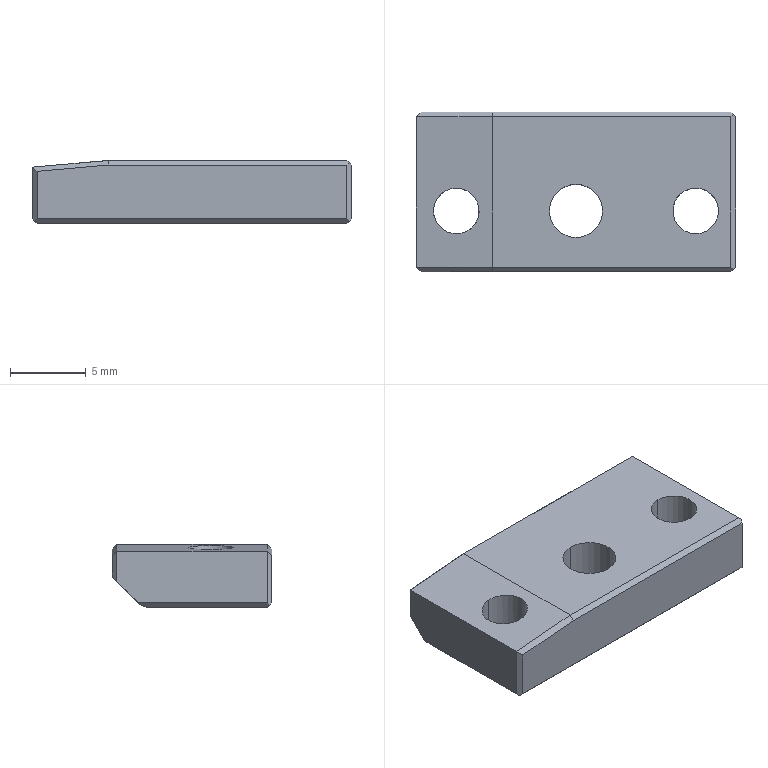Part | NX | 1 solid | 27 faces | box 21 x 10.5 x 4.15 mm | volume 759.288 mm3 | plane 21 | cylinder 6 | commonest cylinder face diameters 3 x4 3.5 x2
STEP:
#1=CARTESIAN_POINT('',(-121.3,173.5,-96.5));
#2=VERTEX_POINT('',#1);
#3=CARTESIAN_POINT('',(-137.,173.5,-96.5));
#4=VERTEX_POINT('',#3);
#5=CARTESIAN_POINT('',(-129.,173.5,-96.5));
#6=DIRECTION('',(-1.,0.,0.));
#7=VECTOR('',#6,1000.);
#8=LINE('',#5,#7);
#9=EDGE_CURVE('',#2,#4,#8,.T.);
#10=ORIENTED_EDGE('',*,*,#9,.F.);
#11=CARTESIAN_POINT('',(-121.3,183.4,-96.5));
#12=VERTEX_POINT('',#11);
#13=CARTESIAN_POINT('',(-121.3,178.45,-96.5));
#14=DIRECTION('',(0.,-1.,0.));
#15=VECTOR('',#14,1000.);
#16=LINE('',#13,#15);
#17=EDGE_CURVE('',#12,#2,#16,.T.);
#18=ORIENTED_EDGE('',*,*,#17,.F.);
#19=CARTESIAN_POINT('',(-137.,183.4,-96.5));
#20=VERTEX_POINT('',#19);
#21=CARTESIAN_POINT('',(-129.,183.4,-96.5));
#22=DIRECTION('',(-1.,0.,0.));
#23=VECTOR('',#22,1000.);
#24=LINE('',#21,#23);
#25=EDGE_CURVE('',#12,#20,#24,.T.);
#26=ORIENTED_EDGE('',*,*,#25,.T.);
#27=CARTESIAN_POINT('',(-137.,178.45,-96.5));
#28=DIRECTION('',(0.,-1.,0.));
#29=VECTOR('',#28,1000.);
#30=LINE('',#27,#29);
#31=EDGE_CURVE('',#20,#4,#30,.T.);
#32=ORIENTED_EDGE('',*,*,#31,.T.);
#33=EDGE_LOOP('',(#10,#18,#26,#32));
#34=FACE_BOUND('',#33,.T.);
#35=CARTESIAN_POINT('',(-123.625,178.7,-96.5));
#36=VERTEX_POINT('',#35);
#37=CARTESIAN_POINT('',(-123.625,175.7,-96.5));
#38=VERTEX_POINT('',#37);
#39=CARTESIAN_POINT('',(-123.625,177.2,-96.5));
#40=DIRECTION('',(0.,0.,-1.));
#41=DIRECTION('',(0.,-1.,0.));
#42=AXIS2_PLACEMENT_3D('',#39,#40,#41);
#43=CIRCLE('',#42,1.5);
#44=EDGE_CURVE('',#36,#38,#43,.T.);
#45=ORIENTED_EDGE('',*,*,#44,.T.);
#46=CARTESIAN_POINT('',(-123.625,177.2,-96.5));
#47=DIRECTION('',(0.,0.,-1.));
#48=DIRECTION('',(0.,-1.,0.));
#49=AXIS2_PLACEMENT_3D('',#46,#47,#48);
#50=CIRCLE('',#49,1.5);
#51=EDGE_CURVE('',#38,#36,#50,.T.);
#52=ORIENTED_EDGE('',*,*,#51,.T.);
#53=EDGE_LOOP('',(#45,#52));
#54=FACE_BOUND('',#53,.T.);
#55=CARTESIAN_POINT('',(-131.5,178.95,-96.5));
#56=VERTEX_POINT('',#55);
#57=CARTESIAN_POINT('',(-131.5,175.45,-96.5));
#58=VERTEX_POINT('',#57);
#59=CARTESIAN_POINT('',(-131.5,177.2,-96.5));
#60=DIRECTION('',(0.,0.,-1.));
#61=DIRECTION('',(0.,-1.,0.));
#62=AXIS2_PLACEMENT_3D('',#59,#60,#61);
#63=CIRCLE('',#62,1.75);
#64=EDGE_CURVE('',#56,#58,#63,.T.);
#65=ORIENTED_EDGE('',*,*,#64,.T.);
#66=CARTESIAN_POINT('',(-131.5,177.2,-96.5));
#67=DIRECTION('',(0.,0.,-1.));
#68=DIRECTION('',(0.,-1.,0.));
#69=AXIS2_PLACEMENT_3D('',#66,#67,#68);
#70=CIRCLE('',#69,1.75);
#71=EDGE_CURVE('',#58,#56,#70,.T.);
#72=ORIENTED_EDGE('',*,*,#71,.T.);
#73=EDGE_LOOP('',(#65,#72));
#74=FACE_BOUND('',#73,.T.);
#75=CARTESIAN_POINT('',(-121.,182.7,-96.5));
#76=DIRECTION('',(0.,0.,1.));
#77=DIRECTION('',(1.,0.,0.));
#78=AXIS2_PLACEMENT_3D('',#75,#76,#77);
#79=PLANE('',#78);
#80=ADVANCED_FACE('',(#34,#54,#74),#79,.T.);
#81=CARTESIAN_POINT('',(-141.7,183.7,-98.65));
#82=VERTEX_POINT('',#81);
#83=CARTESIAN_POINT('',(-121.3,183.7,-98.65));
#84=VERTEX_POINT('',#83);
#85=CARTESIAN_POINT('',(-131.5,183.7,-98.65));
#86=DIRECTION('',(1.,0.,0.));
#87=VECTOR('',#86,1000.);
#88=LINE('',#85,#87);
#89=EDGE_CURVE('',#82,#84,#88,.T.);
#90=ORIENTED_EDGE('',*,*,#89,.F.);
#91=CARTESIAN_POINT('',(-141.7,183.7,-97.212));
#92=VERTEX_POINT('',#91);
#93=CARTESIAN_POINT('',(-141.7,183.7,-97.944));
#94=DIRECTION('',(0.,0.,1.));
#95=VECTOR('',#94,1000.);
#96=LINE('',#93,#95);
#97=EDGE_CURVE('',#82,#92,#96,.T.);
#98=ORIENTED_EDGE('',*,*,#97,.T.);
#99=CARTESIAN_POINT('',(-136.987,183.7,-96.8));
#100=VERTEX_POINT('',#99);
#101=CARTESIAN_POINT('',(-139.474,183.7,-97.018));
#102=DIRECTION('',(0.9962,0.,0.08716));
#103=VECTOR('',#102,1000.);
#104=LINE('',#101,#103);
#105=EDGE_CURVE('',#92,#100,#104,.T.);
#106=ORIENTED_EDGE('',*,*,#105,.T.);
#107=CARTESIAN_POINT('',(-121.3,183.7,-96.8));
#108=VERTEX_POINT('',#107);
#109=CARTESIAN_POINT('',(-129.,183.7,-96.8));
#110=DIRECTION('',(-1.,0.,0.));
#111=VECTOR('',#110,1000.);
#112=LINE('',#109,#111);
#113=EDGE_CURVE('',#108,#100,#112,.T.);
#114=ORIENTED_EDGE('',*,*,#113,.F.);
#115=CARTESIAN_POINT('',(-121.3,183.7,-97.575));
#116=DIRECTION('',(0.,0.,1.));
#117=VECTOR('',#116,1000.);
#118=LINE('',#115,#117);
#119=EDGE_CURVE('',#84,#108,#118,.T.);
#120=ORIENTED_EDGE('',*,*,#119,.F.);
#121=EDGE_LOOP('',(#90,#98,#106,#114,#120));
#122=FACE_BOUND('',#121,.T.);
#123=CARTESIAN_POINT('',(-121.,183.7,-100.65));
#124=DIRECTION('',(0.,1.,0.));
#125=DIRECTION('',(1.,0.,0.));
#126=AXIS2_PLACEMENT_3D('',#123,#124,#125);
#127=PLANE('',#126);
#128=ADVANCED_FACE('',(#122),#127,.T.);
#129=CARTESIAN_POINT('',(-121.3,173.5,-100.65));
#130=VERTEX_POINT('',#129);
#131=CARTESIAN_POINT('',(-141.7,173.5,-100.65));
#132=VERTEX_POINT('',#131);
#133=CARTESIAN_POINT('',(-131.5,173.5,-100.65));
#134=DIRECTION('',(-1.,0.,0.));
#135=VECTOR('',#134,1000.);
#136=LINE('',#133,#135);
#137=EDGE_CURVE('',#130,#132,#136,.T.);
#138=ORIENTED_EDGE('',*,*,#137,.T.);
#139=CARTESIAN_POINT('',(-141.7,181.4,-100.65));
#140=VERTEX_POINT('',#139);
#141=CARTESIAN_POINT('',(-141.7,177.45,-100.65));
#142=DIRECTION('',(0.,1.,0.));
#143=VECTOR('',#142,1000.);
#144=LINE('',#141,#143);
#145=EDGE_CURVE('',#132,#140,#144,.T.);
#146=ORIENTED_EDGE('',*,*,#145,.T.);
#147=CARTESIAN_POINT('',(-121.3,181.4,-100.65));
#148=VERTEX_POINT('',#147);
#149=CARTESIAN_POINT('',(-131.5,181.4,-100.65));
#150=DIRECTION('',(1.,0.,0.));
#151=VECTOR('',#150,1000.);
#152=LINE('',#149,#151);
#153=EDGE_CURVE('',#140,#148,#152,.T.);
#154=ORIENTED_EDGE('',*,*,#153,.T.);
#155=CARTESIAN_POINT('',(-121.3,177.45,-100.65));
#156=DIRECTION('',(0.,1.,0.));
#157=VECTOR('',#156,1000.);
#158=LINE('',#155,#157);
#159=EDGE_CURVE('',#130,#148,#158,.T.);
#160=ORIENTED_EDGE('',*,*,#159,.F.);
#161=EDGE_LOOP('',(#138,#146,#154,#160));
#162=FACE_BOUND('',#161,.T.);
#163=CARTESIAN_POINT('',(-123.625,178.7,-100.65));
#164=VERTEX_POINT('',#163);
#165=CARTESIAN_POINT('',(-123.625,175.7,-100.65));
#166=VERTEX_POINT('',#165);
#167=CARTESIAN_POINT('',(-123.625,177.2,-100.65));
#168=DIRECTION('',(0.,0.,-1.));
#169=DIRECTION('',(0.,-1.,0.));
#170=AXIS2_PLACEMENT_3D('',#167,#168,#169);
#171=CIRCLE('',#170,1.5);
#172=EDGE_CURVE('',#164,#166,#171,.T.);
#173=ORIENTED_EDGE('',*,*,#172,.F.);
#174=CARTESIAN_POINT('',(-123.625,177.2,-100.65));
#175=DIRECTION('',(0.,0.,-1.));
#176=DIRECTION('',(0.,-1.,0.));
#177=AXIS2_PLACEMENT_3D('',#174,#175,#176);
#178=CIRCLE('',#177,1.5);
#179=EDGE_CURVE('',#166,#164,#178,.T.);
#180=ORIENTED_EDGE('',*,*,#179,.F.);
#181=EDGE_LOOP('',(#173,#180));
#182=FACE_BOUND('',#181,.T.);
#183=CARTESIAN_POINT('',(-139.375,178.7,-100.65));
#184=VERTEX_POINT('',#183);
#185=CARTESIAN_POINT('',(-139.375,175.7,-100.65));
#186=VERTEX_POINT('',#185);
#187=CARTESIAN_POINT('',(-139.375,177.2,-100.65));
#188=DIRECTION('',(0.,0.,-1.));
#189=DIRECTION('',(0.,-1.,0.));
#190=AXIS2_PLACEMENT_3D('',#187,#188,#189);
#191=CIRCLE('',#190,1.5);
#192=EDGE_CURVE('',#184,#186,#191,.T.);
#193=ORIENTED_EDGE('',*,*,#192,.F.);
#194=CARTESIAN_POINT('',(-139.375,177.2,-100.65));
#195=DIRECTION('',(0.,0.,-1.));
#196=DIRECTION('',(0.,-1.,0.));
#197=AXIS2_PLACEMENT_3D('',#194,#195,#196);
#198=CIRCLE('',#197,1.5);
#199=EDGE_CURVE('',#186,#184,#198,.T.);
#200=ORIENTED_EDGE('',*,*,#199,.F.);
#201=EDGE_LOOP('',(#193,#200));
#202=FACE_BOUND('',#201,.T.);
#203=CARTESIAN_POINT('',(-131.5,178.95,-100.65));
#204=VERTEX_POINT('',#203);
#205=CARTESIAN_POINT('',(-131.5,175.45,-100.65));
#206=VERTEX_POINT('',#205);
#207=CARTESIAN_POINT('',(-131.5,177.2,-100.65));
#208=DIRECTION('',(0.,0.,-1.));
#209=DIRECTION('',(0.,-1.,0.));
#210=AXIS2_PLACEMENT_3D('',#207,#208,#209);
#211=CIRCLE('',#210,1.75);
#212=EDGE_CURVE('',#204,#206,#211,.T.);
#213=ORIENTED_EDGE('',*,*,#212,.F.);
#214=CARTESIAN_POINT('',(-131.5,177.2,-100.65));
#215=DIRECTION('',(0.,0.,-1.));
#216=DIRECTION('',(0.,-1.,0.));
#217=AXIS2_PLACEMENT_3D('',#214,#215,#216);
#218=CIRCLE('',#217,1.75);
#219=EDGE_CURVE('',#206,#204,#218,.T.);
#220=ORIENTED_EDGE('',*,*,#219,.F.);
#221=EDGE_LOOP('',(#213,#220));
#222=FACE_BOUND('',#221,.T.);
#223=CARTESIAN_POINT('',(-121.,173.2,-100.65));
#224=DIRECTION('',(0.,0.,-1.));
#225=DIRECTION('',(0.,-1.,0.));
#226=AXIS2_PLACEMENT_3D('',#223,#224,#225);
#227=PLANE('',#226);
#228=ADVANCED_FACE('',(#162,#182,#202,#222),#227,.T.);
#229=CARTESIAN_POINT('',(-121.3,173.2,-96.8));
#230=VERTEX_POINT('',#229);
#231=CARTESIAN_POINT('',(-121.3,173.2,-100.35));
#232=VERTEX_POINT('',#231);
#233=CARTESIAN_POINT('',(-121.3,173.2,-98.575));
#234=DIRECTION('',(0.,0.,-1.));
#235=VECTOR('',#234,1000.);
#236=LINE('',#233,#235);
#237=EDGE_CURVE('',#230,#232,#236,.T.);
#238=ORIENTED_EDGE('',*,*,#237,.F.);
#239=CARTESIAN_POINT('',(-136.987,173.2,-96.8));
#240=VERTEX_POINT('',#239);
#241=CARTESIAN_POINT('',(-129.,173.2,-96.8));
#242=DIRECTION('',(-1.,0.,0.));
#243=VECTOR('',#242,1000.);
#244=LINE('',#241,#243);
#245=EDGE_CURVE('',#230,#240,#244,.T.);
#246=ORIENTED_EDGE('',*,*,#245,.T.);
#247=CARTESIAN_POINT('',(-141.7,173.2,-97.212));
#248=VERTEX_POINT('',#247);
#249=CARTESIAN_POINT('',(-139.474,173.2,-97.018));
#250=DIRECTION('',(-0.9962,0.,-0.08716));
#251=VECTOR('',#250,1000.);
#252=LINE('',#249,#251);
#253=EDGE_CURVE('',#240,#248,#252,.T.);
#254=ORIENTED_EDGE('',*,*,#253,.T.);
#255=CARTESIAN_POINT('',(-141.7,173.2,-100.35));
#256=VERTEX_POINT('',#255);
#257=CARTESIAN_POINT('',(-141.7,173.2,-98.794));
#258=DIRECTION('',(0.,0.,-1.));
#259=VECTOR('',#258,1000.);
#260=LINE('',#257,#259);
#261=EDGE_CURVE('',#248,#256,#260,.T.);
#262=ORIENTED_EDGE('',*,*,#261,.T.);
#263=CARTESIAN_POINT('',(-131.5,173.2,-100.35));
#264=DIRECTION('',(-1.,0.,0.));
#265=VECTOR('',#264,1000.);
#266=LINE('',#263,#265);
#267=EDGE_CURVE('',#232,#256,#266,.T.);
#268=ORIENTED_EDGE('',*,*,#267,.F.);
#269=EDGE_LOOP('',(#238,#246,#254,#262,#268));
#270=FACE_BOUND('',#269,.T.);
#271=CARTESIAN_POINT('',(-121.,173.2,-96.5));
#272=DIRECTION('',(0.,-1.,0.));
#273=DIRECTION('',(0.,0.,-1.));
#274=AXIS2_PLACEMENT_3D('',#271,#272,#273);
#275=PLANE('',#274);
#276=ADVANCED_FACE('',(#270),#275,.T.);
#277=CARTESIAN_POINT('',(-141.912,181.912,-100.438));
#278=VERTEX_POINT('',#277);
#279=CARTESIAN_POINT('',(-121.088,181.912,-100.438));
#280=VERTEX_POINT('',#279);
#281=CARTESIAN_POINT('',(-131.5,181.912,-100.438));
#282=DIRECTION('',(1.,0.,0.));
#283=VECTOR('',#282,1000.);
#284=LINE('',#281,#283);
#285=EDGE_CURVE('',#278,#280,#284,.T.);
#286=ORIENTED_EDGE('',*,*,#285,.F.);
#287=CARTESIAN_POINT('',(-142.,182.,-100.35));
#288=VERTEX_POINT('',#287);
#289=CARTESIAN_POINT('',(-121.,161.,-121.35));
#290=DIRECTION('',(0.5774,-0.5774,-0.5774));
#291=VECTOR('',#290,1000.);
#292=LINE('',#289,#291);
#293=EDGE_CURVE('',#288,#278,#292,.T.);
#294=ORIENTED_EDGE('',*,*,#293,.F.);
#295=CARTESIAN_POINT('',(-142.,183.4,-98.95));
#296=VERTEX_POINT('',#295);
#297=CARTESIAN_POINT('',(-142.,196.267,-86.083));
#298=DIRECTION('',(0.,0.7071,0.7071));
#299=VECTOR('',#298,1000.);
#300=LINE('',#297,#299);
#301=EDGE_CURVE('',#288,#296,#300,.T.);
#302=ORIENTED_EDGE('',*,*,#301,.T.);
#303=CARTESIAN_POINT('',(-121.,204.4,-77.95));
#304=DIRECTION('',(-0.5774,-0.5774,-0.5774));
#305=VECTOR('',#304,1000.);
#306=LINE('',#303,#305);
#307=EDGE_CURVE('',#82,#296,#306,.T.);
#308=ORIENTED_EDGE('',*,*,#307,.F.);
#309=ORIENTED_EDGE('',*,*,#89,.T.);
#310=CARTESIAN_POINT('',(-121.,183.4,-98.95));
#311=VERTEX_POINT('',#310);
#312=CARTESIAN_POINT('',(-121.,183.4,-98.95));
#313=DIRECTION('',(0.5774,-0.5774,-0.5774));
#314=VECTOR('',#313,1000.);
#315=LINE('',#312,#314);
#316=EDGE_CURVE('',#84,#311,#315,.T.);
#317=ORIENTED_EDGE('',*,*,#316,.T.);
#318=CARTESIAN_POINT('',(-121.,182.,-100.35));
#319=VERTEX_POINT('',#318);
#320=CARTESIAN_POINT('',(-121.,196.267,-86.083));
#321=DIRECTION('',(0.,0.7071,0.7071));
#322=VECTOR('',#321,1000.);
#323=LINE('',#320,#322);
#324=EDGE_CURVE('',#319,#311,#323,.T.);
#325=ORIENTED_EDGE('',*,*,#324,.F.);
#326=CARTESIAN_POINT('',(-106.733,196.267,-86.083));
#327=DIRECTION('',(-0.5774,-0.5774,-0.5774));
#328=VECTOR('',#327,1000.);
#329=LINE('',#326,#328);
#330=EDGE_CURVE('',#319,#280,#329,.T.);
#331=ORIENTED_EDGE('',*,*,#330,.T.);
#332=EDGE_LOOP('',(#286,#294,#302,#308,#309,#317,#325,#331));
#333=FACE_BOUND('',#332,.T.);
#334=CARTESIAN_POINT('',(-131.5,182.7,-99.65));
#335=DIRECTION('',(0.,-0.7071,0.7071));
#336=DIRECTION('',(-1.,0.,0.));
#337=AXIS2_PLACEMENT_3D('',#334,#335,#336);
#338=PLANE('',#337);
#339=ADVANCED_FACE('',(#333),#338,.F.);
#340=ORIENTED_EDGE('',*,*,#64,.F.);
#341=CARTESIAN_POINT('',(-131.5,178.95,-96.085));
#342=DIRECTION('',(0.,0.,-1.));
#343=VECTOR('',#342,1000.);
#344=LINE('',#341,#343);
#345=EDGE_CURVE('',#204,#56,#344,.F.);
#346=ORIENTED_EDGE('',*,*,#345,.F.);
#347=ORIENTED_EDGE('',*,*,#212,.T.);
#348=CARTESIAN_POINT('',(-131.5,175.45,-96.085));
#349=DIRECTION('',(0.,0.,-1.));
#350=VECTOR('',#349,1000.);
#351=LINE('',#348,#350);
#352=EDGE_CURVE('',#206,#58,#351,.F.);
#353=ORIENTED_EDGE('',*,*,#352,.T.);
#354=EDGE_LOOP('',(#340,#346,#347,#353));
#355=FACE_BOUND('',#354,.T.);
#356=CARTESIAN_POINT('',(-131.5,177.2,-96.085));
#357=DIRECTION('',(0.,0.,-1.));
#358=DIRECTION('',(0.,-1.,0.));
#359=AXIS2_PLACEMENT_3D('',#356,#357,#358);
#360=CYLINDRICAL_SURFACE('',#359,1.75);
#361=ADVANCED_FACE('',(#355),#360,.F.);
#362=ORIENTED_EDGE('',*,*,#44,.F.);
#363=CARTESIAN_POINT('',(-123.625,178.7,-96.085));
#364=DIRECTION('',(0.,0.,-1.));
#365=VECTOR('',#364,1000.);
#366=LINE('',#363,#365);
#367=EDGE_CURVE('',#164,#36,#366,.F.);
#368=ORIENTED_EDGE('',*,*,#367,.F.);
#369=ORIENTED_EDGE('',*,*,#172,.T.);
#370=CARTESIAN_POINT('',(-123.625,175.7,-96.085));
#371=DIRECTION('',(0.,0.,-1.));
#372=VECTOR('',#371,1000.);
#373=LINE('',#370,#372);
#374=EDGE_CURVE('',#166,#38,#373,.F.);
#375=ORIENTED_EDGE('',*,*,#374,.T.);
#376=EDGE_LOOP('',(#362,#368,#369,#375));
#377=FACE_BOUND('',#376,.T.);
#378=CARTESIAN_POINT('',(-123.625,177.2,-96.085));
#379=DIRECTION('',(0.,0.,-1.));
#380=DIRECTION('',(0.,-1.,0.));
#381=AXIS2_PLACEMENT_3D('',#378,#379,#380);
#382=CYLINDRICAL_SURFACE('',#381,1.5);
#383=ADVANCED_FACE('',(#377),#382,.F.);
#384=CARTESIAN_POINT('',(-139.375,178.7,-96.708));
#385=VERTEX_POINT('',#384);
#386=CARTESIAN_POINT('',(-139.375,175.7,-96.708));
#387=VERTEX_POINT('',#386);
#388=CARTESIAN_POINT('',(-139.375,178.7,-96.708));
#389=CARTESIAN_POINT('',(-136.375,178.7,-96.445));
#390=CARTESIAN_POINT('',(-136.375,175.7,-96.445));
#391=CARTESIAN_POINT('',(-139.375,175.7,-96.708));
#392=(BOUNDED_CURVE()B_SPLINE_CURVE(3,(#388,#389,#390,#391),.UNSPECIFIED.,.F.,.F.)B_SPLINE_CURVE_WITH_KNOTS((4,4),(4.712,7.854),.UNSPECIFIED.)CURVE()GEOMETRIC_REPRESENTATION_ITEM()RATIONAL_B_SPLINE_CURVE((1.,0.3333,0.3333,1.))REPRESENTATION_ITEM(''));
#393=EDGE_CURVE('',#385,#387,#392,.T.);
#394=ORIENTED_EDGE('',*,*,#393,.F.);
#395=CARTESIAN_POINT('',(-139.375,178.7,-96.085));
#396=DIRECTION('',(0.,0.,-1.));
#397=VECTOR('',#396,1000.);
#398=LINE('',#395,#397);
#399=EDGE_CURVE('',#184,#385,#398,.F.);
#400=ORIENTED_EDGE('',*,*,#399,.F.);
#401=ORIENTED_EDGE('',*,*,#192,.T.);
#402=CARTESIAN_POINT('',(-139.375,175.7,-96.085));
#403=DIRECTION('',(0.,0.,-1.));
#404=VECTOR('',#403,1000.);
#405=LINE('',#402,#404);
#406=EDGE_CURVE('',#186,#387,#405,.F.);
#407=ORIENTED_EDGE('',*,*,#406,.T.);
#408=EDGE_LOOP('',(#394,#400,#401,#407));
#409=FACE_BOUND('',#408,.T.);
#410=CARTESIAN_POINT('',(-139.375,177.2,-96.085));
#411=DIRECTION('',(0.,0.,-1.));
#412=DIRECTION('',(0.,-1.,0.));
#413=AXIS2_PLACEMENT_3D('',#410,#411,#412);
#414=CYLINDRICAL_SURFACE('',#413,1.5);
#415=ADVANCED_FACE('',(#409),#414,.F.);
#416=ORIENTED_EDGE('',*,*,#25,.F.);
#417=CARTESIAN_POINT('',(-121.15,183.55,-96.65));
#418=VERTEX_POINT('',#417);
#419=CARTESIAN_POINT('',(-131.717,172.983,-86.083));
#420=DIRECTION('',(0.5774,0.5774,-0.5774));
#421=VECTOR('',#420,1000.);
#422=LINE('',#419,#421);
#423=EDGE_CURVE('',#12,#418,#422,.T.);
#424=ORIENTED_EDGE('',*,*,#423,.T.);
#425=CARTESIAN_POINT('',(-110.583,172.983,-86.083));
#426=DIRECTION('',(-0.5774,0.5774,-0.5774));
#427=VECTOR('',#426,1000.);
#428=LINE('',#425,#427);
#429=EDGE_CURVE('',#418,#108,#428,.T.);
#430=ORIENTED_EDGE('',*,*,#429,.T.);
#431=ORIENTED_EDGE('',*,*,#113,.T.);
#432=CARTESIAN_POINT('',(-137.455,172.983,-86.083));
#433=DIRECTION('',(0.03086,0.7068,-0.7068));
#434=VECTOR('',#433,1000.);
#435=LINE('',#432,#434);
#436=EDGE_CURVE('',#20,#100,#435,.T.);
#437=ORIENTED_EDGE('',*,*,#436,.F.);
#438=EDGE_LOOP('',(#416,#424,#430,#431,#437));
#439=FACE_BOUND('',#438,.T.);
#440=CARTESIAN_POINT('',(-129.,183.55,-96.65));
#441=DIRECTION('',(0.,0.7071,0.7071));
#442=DIRECTION('',(1.,0.,0.));
#443=AXIS2_PLACEMENT_3D('',#440,#441,#442);
#444=PLANE('',#443);
#445=ADVANCED_FACE('',(#439),#444,.T.);
#446=ORIENTED_EDGE('',*,*,#285,.T.);
#447=CARTESIAN_POINT('',(-122.939,177.442,-102.289));
#448=DIRECTION('',(0.3574,0.8629,0.3574));
#449=VECTOR('',#448,1000.);
#450=LINE('',#447,#449);
#451=EDGE_CURVE('',#148,#280,#450,.T.);
#452=ORIENTED_EDGE('',*,*,#451,.F.);
#453=ORIENTED_EDGE('',*,*,#153,.F.);
#454=CARTESIAN_POINT('',(-140.061,177.442,-102.289));
#455=DIRECTION('',(-0.3574,0.8629,0.3574));
#456=VECTOR('',#455,1000.);
#457=LINE('',#454,#456);
#458=EDGE_CURVE('',#140,#278,#457,.T.);
#459=ORIENTED_EDGE('',*,*,#458,.T.);
#460=EDGE_LOOP('',(#446,#452,#453,#459));
#461=FACE_BOUND('',#460,.T.);
#462=CARTESIAN_POINT('',(-131.5,181.656,-100.544));
#463=DIRECTION('',(0.,-0.3827,0.9239));
#464=DIRECTION('',(-1.,0.,0.));
#465=AXIS2_PLACEMENT_3D('',#462,#463,#464);
#466=PLANE('',#465);
#467=ADVANCED_FACE('',(#461),#466,.F.);
#468=ORIENTED_EDGE('',*,*,#137,.F.);
#469=CARTESIAN_POINT('',(-121.15,173.35,-100.5));
#470=VERTEX_POINT('',#469);
#471=CARTESIAN_POINT('',(-106.733,158.933,-86.083));
#472=DIRECTION('',(0.5774,-0.5774,0.5774));
#473=VECTOR('',#472,1000.);
#474=LINE('',#471,#473);
#475=EDGE_CURVE('',#130,#470,#474,.T.);
#476=ORIENTED_EDGE('',*,*,#475,.T.);
#477=CARTESIAN_POINT('',(-135.567,158.933,-86.083));
#478=DIRECTION('',(-0.5774,-0.5774,0.5774));
#479=VECTOR('',#478,1000.);
#480=LINE('',#477,#479);
#481=EDGE_CURVE('',#470,#232,#480,.T.);
#482=ORIENTED_EDGE('',*,*,#481,.T.);
#483=ORIENTED_EDGE('',*,*,#267,.T.);
#484=CARTESIAN_POINT('',(-141.85,173.35,-100.5));
#485=VERTEX_POINT('',#484);
#486=CARTESIAN_POINT('',(-121.,152.5,-79.65));
#487=DIRECTION('',(-0.5774,0.5774,-0.5774));
#488=VECTOR('',#487,1000.);
#489=LINE('',#486,#488);
#490=EDGE_CURVE('',#256,#485,#489,.T.);
#491=ORIENTED_EDGE('',*,*,#490,.T.);
#492=CARTESIAN_POINT('',(-121.,194.2,-121.35));
#493=DIRECTION('',(0.5774,0.5774,-0.5774));
#494=VECTOR('',#493,1000.);
#495=LINE('',#492,#494);
#496=EDGE_CURVE('',#485,#132,#495,.T.);
#497=ORIENTED_EDGE('',*,*,#496,.T.);
#498=EDGE_LOOP('',(#468,#476,#482,#483,#491,#497));
#499=FACE_BOUND('',#498,.T.);
#500=CARTESIAN_POINT('',(-131.5,173.35,-100.5));
#501=DIRECTION('',(0.,-0.7071,-0.7071));
#502=DIRECTION('',(0.,0.7071,-0.7071));
#503=AXIS2_PLACEMENT_3D('',#500,#501,#502);
#504=PLANE('',#503);
#505=ADVANCED_FACE('',(#499),#504,.T.);
#506=ORIENTED_EDGE('',*,*,#9,.T.);
#507=CARTESIAN_POINT('',(-137.455,183.917,-86.083));
#508=DIRECTION('',(0.03086,-0.7068,-0.7068));
#509=VECTOR('',#508,1000.);
#510=LINE('',#507,#509);
#511=EDGE_CURVE('',#4,#240,#510,.T.);
#512=ORIENTED_EDGE('',*,*,#511,.T.);
#513=ORIENTED_EDGE('',*,*,#245,.F.);
#514=CARTESIAN_POINT('',(-121.15,173.35,-96.65));
#515=VERTEX_POINT('',#514);
#516=CARTESIAN_POINT('',(-121.,173.5,-96.5));
#517=DIRECTION('',(-0.5774,-0.5774,-0.5774));
#518=VECTOR('',#517,1000.);
#519=LINE('',#516,#518);
#520=EDGE_CURVE('',#515,#230,#519,.T.);
#521=ORIENTED_EDGE('',*,*,#520,.F.);
#522=CARTESIAN_POINT('',(-131.717,183.917,-86.083));
#523=DIRECTION('',(0.5774,-0.5774,-0.5774));
#524=VECTOR('',#523,1000.);
#525=LINE('',#522,#524);
#526=EDGE_CURVE('',#2,#515,#525,.T.);
#527=ORIENTED_EDGE('',*,*,#526,.F.);
#528=EDGE_LOOP('',(#506,#512,#513,#521,#527));
#529=FACE_BOUND('',#528,.T.);
#530=CARTESIAN_POINT('',(-129.,173.35,-96.65));
#531=DIRECTION('',(0.,0.7071,-0.7071));
#532=DIRECTION('',(-1.,0.,0.));
#533=AXIS2_PLACEMENT_3D('',#530,#531,#532);
#534=PLANE('',#533);
#535=ADVANCED_FACE('',(#529),#534,.F.);
#536=ORIENTED_EDGE('',*,*,#406,.F.);
#537=ORIENTED_EDGE('',*,*,#199,.T.);
#538=ORIENTED_EDGE('',*,*,#399,.T.);
#539=CARTESIAN_POINT('',(-139.375,175.7,-96.708));
#540=CARTESIAN_POINT('',(-142.375,175.7,-96.97));
#541=CARTESIAN_POINT('',(-142.375,178.7,-96.97));
#542=CARTESIAN_POINT('',(-139.375,178.7,-96.708));
#543=(BOUNDED_CURVE()B_SPLINE_CURVE(3,(#539,#540,#541,#542),.UNSPECIFIED.,.F.,.F.)B_SPLINE_CURVE_WITH_KNOTS((4,4),(1.571,4.712),.UNSPECIFIED.)CURVE()GEOMETRIC_REPRESENTATION_ITEM()RATIONAL_B_SPLINE_CURVE((1.,0.3333,0.3333,1.))REPRESENTATION_ITEM(''));
#544=EDGE_CURVE('',#387,#385,#543,.T.);
#545=ORIENTED_EDGE('',*,*,#544,.F.);
#546=EDGE_LOOP('',(#536,#537,#538,#545));
#547=FACE_BOUND('',#546,.T.);
#548=CARTESIAN_POINT('',(-139.375,177.2,-96.085));
#549=DIRECTION('',(0.,0.,-1.));
#550=DIRECTION('',(0.,-1.,0.));
#551=AXIS2_PLACEMENT_3D('',#548,#549,#550);
#552=CYLINDRICAL_SURFACE('',#551,1.5);
#553=ADVANCED_FACE('',(#547),#552,.F.);
#554=ORIENTED_EDGE('',*,*,#374,.F.);
#555=ORIENTED_EDGE('',*,*,#179,.T.);
#556=ORIENTED_EDGE('',*,*,#367,.T.);
#557=ORIENTED_EDGE('',*,*,#51,.F.);
#558=EDGE_LOOP('',(#554,#555,#556,#557));
#559=FACE_BOUND('',#558,.T.);
#560=CARTESIAN_POINT('',(-123.625,177.2,-96.085));
#561=DIRECTION('',(0.,0.,-1.));
#562=DIRECTION('',(0.,-1.,0.));
#563=AXIS2_PLACEMENT_3D('',#560,#561,#562);
#564=CYLINDRICAL_SURFACE('',#563,1.5);
#565=ADVANCED_FACE('',(#559),#564,.F.);
#566=ORIENTED_EDGE('',*,*,#352,.F.);
#567=ORIENTED_EDGE('',*,*,#219,.T.);
#568=ORIENTED_EDGE('',*,*,#345,.T.);
#569=ORIENTED_EDGE('',*,*,#71,.F.);
#570=EDGE_LOOP('',(#566,#567,#568,#569));
#571=FACE_BOUND('',#570,.T.);
#572=CARTESIAN_POINT('',(-131.5,177.2,-96.085));
#573=DIRECTION('',(0.,0.,-1.));
#574=DIRECTION('',(0.,-1.,0.));
#575=AXIS2_PLACEMENT_3D('',#572,#573,#574);
#576=CYLINDRICAL_SURFACE('',#575,1.75);
#577=ADVANCED_FACE('',(#571),#576,.F.);
#578=CARTESIAN_POINT('',(-142.,183.4,-96.937));
#579=VERTEX_POINT('',#578);
#580=CARTESIAN_POINT('',(-142.,183.4,-97.944));
#581=DIRECTION('',(0.,0.,1.));
#582=VECTOR('',#581,1000.);
#583=LINE('',#580,#582);
#584=EDGE_CURVE('',#296,#579,#583,.T.);
#585=ORIENTED_EDGE('',*,*,#584,.F.);
#586=ORIENTED_EDGE('',*,*,#301,.F.);
#587=CARTESIAN_POINT('',(-142.,173.5,-100.35));
#588=VERTEX_POINT('',#587);
#589=CARTESIAN_POINT('',(-142.,177.45,-100.35));
#590=DIRECTION('',(0.,1.,0.));
#591=VECTOR('',#590,1000.);
#592=LINE('',#589,#591);
#593=EDGE_CURVE('',#588,#288,#592,.T.);
#594=ORIENTED_EDGE('',*,*,#593,.F.);
#595=CARTESIAN_POINT('',(-142.,173.5,-96.937));
#596=VERTEX_POINT('',#595);
#597=CARTESIAN_POINT('',(-142.,173.5,-98.794));
#598=DIRECTION('',(0.,0.,-1.));
#599=VECTOR('',#598,1000.);
#600=LINE('',#597,#599);
#601=EDGE_CURVE('',#596,#588,#600,.T.);
#602=ORIENTED_EDGE('',*,*,#601,.F.);
#603=CARTESIAN_POINT('',(-142.,178.45,-96.937));
#604=DIRECTION('',(0.,-1.,0.));
#605=VECTOR('',#604,1000.);
#606=LINE('',#603,#605);
#607=EDGE_CURVE('',#579,#596,#606,.T.);
#608=ORIENTED_EDGE('',*,*,#607,.F.);
#609=EDGE_LOOP('',(#585,#586,#594,#602,#608));
#610=FACE_BOUND('',#609,.T.);
#611=CARTESIAN_POINT('',(-142.,177.442,-86.083));
#612=DIRECTION('',(1.,0.,0.));
#613=DIRECTION('',(0.,1.,0.));
#614=AXIS2_PLACEMENT_3D('',#611,#612,#613);
#615=PLANE('',#614);
#616=ADVANCED_FACE('',(#610),#615,.F.);
#617=CARTESIAN_POINT('',(-139.5,173.5,-96.719));
#618=DIRECTION('',(-0.9962,0.,-0.08716));
#619=VECTOR('',#618,1000.);
#620=LINE('',#617,#619);
#621=EDGE_CURVE('',#4,#596,#620,.T.);
#622=ORIENTED_EDGE('',*,*,#621,.F.);
#623=ORIENTED_EDGE('',*,*,#31,.F.);
#624=CARTESIAN_POINT('',(-139.5,183.4,-96.719));
#625=DIRECTION('',(0.9962,0.,0.08716));
#626=VECTOR('',#625,1000.);
#627=LINE('',#624,#626);
#628=EDGE_CURVE('',#579,#20,#627,.T.);
#629=ORIENTED_EDGE('',*,*,#628,.F.);
#630=ORIENTED_EDGE('',*,*,#607,.T.);
#631=EDGE_LOOP('',(#622,#623,#629,#630));
#632=FACE_BOUND('',#631,.T.);
#633=ORIENTED_EDGE('',*,*,#393,.T.);
#634=ORIENTED_EDGE('',*,*,#544,.T.);
#635=EDGE_LOOP('',(#633,#634));
#636=FACE_BOUND('',#635,.T.);
#637=CARTESIAN_POINT('',(-139.5,178.45,-96.719));
#638=DIRECTION('',(0.08716,0.,-0.9962));
#639=DIRECTION('',(0.,-1.,0.));
#640=AXIS2_PLACEMENT_3D('',#637,#638,#639);
#641=PLANE('',#640);
#642=ADVANCED_FACE('',(#632,#636),#641,.F.);
#643=ORIENTED_EDGE('',*,*,#628,.T.);
#644=ORIENTED_EDGE('',*,*,#436,.T.);
#645=ORIENTED_EDGE('',*,*,#105,.F.);
#646=CARTESIAN_POINT('',(-121.,204.4,-116.18));
#647=DIRECTION('',(0.5934,0.5934,-0.5438));
#648=VECTOR('',#647,1000.);
#649=LINE('',#646,#648);
#650=EDGE_CURVE('',#579,#92,#649,.T.);
#651=ORIENTED_EDGE('',*,*,#650,.F.);
#652=EDGE_LOOP('',(#643,#644,#645,#651));
#653=FACE_BOUND('',#652,.T.);
#654=CARTESIAN_POINT('',(-139.487,183.55,-96.868));
#655=DIRECTION('',(0.06163,-0.7071,-0.7044));
#656=DIRECTION('',(0.,0.7058,-0.7085));
#657=AXIS2_PLACEMENT_3D('',#654,#655,#656);
#658=PLANE('',#657);
#659=ADVANCED_FACE('',(#653),#658,.F.);
#660=ORIENTED_EDGE('',*,*,#593,.T.);
#661=ORIENTED_EDGE('',*,*,#293,.T.);
#662=ORIENTED_EDGE('',*,*,#458,.F.);
#663=ORIENTED_EDGE('',*,*,#145,.F.);
#664=ORIENTED_EDGE('',*,*,#496,.F.);
#665=CARTESIAN_POINT('',(-156.267,187.767,-86.083));
#666=DIRECTION('',(-0.5774,0.5774,0.5774));
#667=VECTOR('',#666,1000.);
#668=LINE('',#665,#667);
#669=EDGE_CURVE('',#485,#588,#668,.T.);
#670=ORIENTED_EDGE('',*,*,#669,.T.);
#671=EDGE_LOOP('',(#660,#661,#662,#663,#664,#670));
#672=FACE_BOUND('',#671,.T.);
#673=CARTESIAN_POINT('',(-141.85,177.45,-100.5));
#674=DIRECTION('',(0.7071,0.,0.7071));
#675=DIRECTION('',(0.,-1.,0.));
#676=AXIS2_PLACEMENT_3D('',#673,#674,#675);
#677=PLANE('',#676);
#678=ADVANCED_FACE('',(#672),#677,.F.);
#679=ORIENTED_EDGE('',*,*,#601,.T.);
#680=ORIENTED_EDGE('',*,*,#669,.F.);
#681=ORIENTED_EDGE('',*,*,#490,.F.);
#682=ORIENTED_EDGE('',*,*,#261,.F.);
#683=CARTESIAN_POINT('',(-121.,152.5,-116.18));
#684=DIRECTION('',(-0.5934,0.5934,0.5438));
#685=VECTOR('',#684,1000.);
#686=LINE('',#683,#685);
#687=EDGE_CURVE('',#248,#596,#686,.T.);
#688=ORIENTED_EDGE('',*,*,#687,.T.);
#689=EDGE_LOOP('',(#679,#680,#681,#682,#688));
#690=FACE_BOUND('',#689,.T.);
#691=CARTESIAN_POINT('',(-141.85,173.35,-98.794));
#692=DIRECTION('',(0.7071,0.7071,0.));
#693=DIRECTION('',(0.,0.,-1.));
#694=AXIS2_PLACEMENT_3D('',#691,#692,#693);
#695=PLANE('',#694);
#696=ADVANCED_FACE('',(#690),#695,.F.);
#697=ORIENTED_EDGE('',*,*,#621,.T.);
#698=ORIENTED_EDGE('',*,*,#687,.F.);
#699=ORIENTED_EDGE('',*,*,#253,.F.);
#700=ORIENTED_EDGE('',*,*,#511,.F.);
#701=EDGE_LOOP('',(#697,#698,#699,#700));
#702=FACE_BOUND('',#701,.T.);
#703=CARTESIAN_POINT('',(-139.487,173.35,-96.868));
#704=DIRECTION('',(0.06163,0.7071,-0.7044));
#705=DIRECTION('',(-0.9962,0.,-0.08716));
#706=AXIS2_PLACEMENT_3D('',#703,#704,#705);
#707=PLANE('',#706);
#708=ADVANCED_FACE('',(#702),#707,.F.);
#709=ORIENTED_EDGE('',*,*,#584,.T.);
#710=ORIENTED_EDGE('',*,*,#650,.T.);
#711=ORIENTED_EDGE('',*,*,#97,.F.);
#712=ORIENTED_EDGE('',*,*,#307,.T.);
#713=EDGE_LOOP('',(#709,#710,#711,#712));
#714=FACE_BOUND('',#713,.T.);
#715=CARTESIAN_POINT('',(-141.85,183.55,-97.944));
#716=DIRECTION('',(0.7071,-0.7071,0.));
#717=DIRECTION('',(0.,0.,-1.));
#718=AXIS2_PLACEMENT_3D('',#715,#716,#717);
#719=PLANE('',#718);
#720=ADVANCED_FACE('',(#714),#719,.F.);
#721=CARTESIAN_POINT('',(-121.,183.4,-96.8));
#722=VERTEX_POINT('',#721);
#723=CARTESIAN_POINT('',(-121.,183.4,-97.575));
#724=DIRECTION('',(0.,0.,1.));
#725=VECTOR('',#724,1000.);
#726=LINE('',#723,#725);
#727=EDGE_CURVE('',#311,#722,#726,.T.);
#728=ORIENTED_EDGE('',*,*,#727,.T.);
#729=CARTESIAN_POINT('',(-121.,173.5,-96.8));
#730=VERTEX_POINT('',#729);
#731=CARTESIAN_POINT('',(-121.,178.45,-96.8));
#732=DIRECTION('',(0.,-1.,0.));
#733=VECTOR('',#732,1000.);
#734=LINE('',#731,#733);
#735=EDGE_CURVE('',#722,#730,#734,.T.);
#736=ORIENTED_EDGE('',*,*,#735,.T.);
#737=CARTESIAN_POINT('',(-121.,173.5,-100.35));
#738=VERTEX_POINT('',#737);
#739=CARTESIAN_POINT('',(-121.,173.5,-98.575));
#740=DIRECTION('',(0.,0.,-1.));
#741=VECTOR('',#740,1000.);
#742=LINE('',#739,#741);
#743=EDGE_CURVE('',#730,#738,#742,.T.);
#744=ORIENTED_EDGE('',*,*,#743,.T.);
#745=CARTESIAN_POINT('',(-121.,177.45,-100.35));
#746=DIRECTION('',(0.,1.,0.));
#747=VECTOR('',#746,1000.);
#748=LINE('',#745,#747);
#749=EDGE_CURVE('',#738,#319,#748,.T.);
#750=ORIENTED_EDGE('',*,*,#749,.T.);
#751=ORIENTED_EDGE('',*,*,#324,.T.);
#752=EDGE_LOOP('',(#728,#736,#744,#750,#751));
#753=FACE_BOUND('',#752,.T.);
#754=CARTESIAN_POINT('',(-121.,177.442,-86.083));
#755=DIRECTION('',(1.,0.,0.));
#756=DIRECTION('',(0.,1.,0.));
#757=AXIS2_PLACEMENT_3D('',#754,#755,#756);
#758=PLANE('',#757);
#759=ADVANCED_FACE('',(#753),#758,.T.);
#760=ORIENTED_EDGE('',*,*,#743,.F.);
#761=CARTESIAN_POINT('',(-131.717,162.783,-86.083));
#762=DIRECTION('',(-0.5774,-0.5774,0.5774));
#763=VECTOR('',#762,1000.);
#764=LINE('',#761,#763);
#765=EDGE_CURVE('',#730,#515,#764,.T.);
#766=ORIENTED_EDGE('',*,*,#765,.T.);
#767=ORIENTED_EDGE('',*,*,#520,.T.);
#768=ORIENTED_EDGE('',*,*,#237,.T.);
#769=ORIENTED_EDGE('',*,*,#481,.F.);
#770=CARTESIAN_POINT('',(-106.733,187.767,-86.083));
#771=DIRECTION('',(0.5774,0.5774,0.5774));
#772=VECTOR('',#771,1000.);
#773=LINE('',#770,#772);
#774=EDGE_CURVE('',#470,#738,#773,.T.);
#775=ORIENTED_EDGE('',*,*,#774,.T.);
#776=EDGE_LOOP('',(#760,#766,#767,#768,#769,#775));
#777=FACE_BOUND('',#776,.T.);
#778=CARTESIAN_POINT('',(-121.15,173.35,-98.575));
#779=DIRECTION('',(0.7071,-0.7071,0.));
#780=DIRECTION('',(0.,0.,-1.));
#781=AXIS2_PLACEMENT_3D('',#778,#779,#780);
#782=PLANE('',#781);
#783=ADVANCED_FACE('',(#777),#782,.T.);
#784=ORIENTED_EDGE('',*,*,#749,.F.);
#785=ORIENTED_EDGE('',*,*,#774,.F.);
#786=ORIENTED_EDGE('',*,*,#475,.F.);
#787=ORIENTED_EDGE('',*,*,#159,.T.);
#788=ORIENTED_EDGE('',*,*,#451,.T.);
#789=ORIENTED_EDGE('',*,*,#330,.F.);
#790=EDGE_LOOP('',(#784,#785,#786,#787,#788,#789));
#791=FACE_BOUND('',#790,.T.);
#792=CARTESIAN_POINT('',(-121.15,177.45,-100.5));
#793=DIRECTION('',(0.7071,0.,-0.7071));
#794=DIRECTION('',(0.,-1.,0.));
#795=AXIS2_PLACEMENT_3D('',#792,#793,#794);
#796=PLANE('',#795);
#797=ADVANCED_FACE('',(#791),#796,.T.);
#798=ORIENTED_EDGE('',*,*,#735,.F.);
#799=CARTESIAN_POINT('',(-131.717,194.117,-86.083));
#800=DIRECTION('',(-0.5774,0.5774,0.5774));
#801=VECTOR('',#800,1000.);
#802=LINE('',#799,#801);
#803=EDGE_CURVE('',#722,#418,#802,.T.);
#804=ORIENTED_EDGE('',*,*,#803,.T.);
#805=ORIENTED_EDGE('',*,*,#423,.F.);
#806=ORIENTED_EDGE('',*,*,#17,.T.);
#807=ORIENTED_EDGE('',*,*,#526,.T.);
#808=ORIENTED_EDGE('',*,*,#765,.F.);
#809=EDGE_LOOP('',(#798,#804,#805,#806,#807,#808));
#810=FACE_BOUND('',#809,.T.);
#811=CARTESIAN_POINT('',(-121.15,178.45,-96.65));
#812=DIRECTION('',(0.7071,0.,0.7071));
#813=DIRECTION('',(0.,-1.,0.));
#814=AXIS2_PLACEMENT_3D('',#811,#812,#813);
#815=PLANE('',#814);
#816=ADVANCED_FACE('',(#810),#815,.T.);
#817=ORIENTED_EDGE('',*,*,#727,.F.);
#818=ORIENTED_EDGE('',*,*,#316,.F.);
#819=ORIENTED_EDGE('',*,*,#119,.T.);
#820=ORIENTED_EDGE('',*,*,#429,.F.);
#821=ORIENTED_EDGE('',*,*,#803,.F.);
#822=EDGE_LOOP('',(#817,#818,#819,#820,#821));
#823=FACE_BOUND('',#822,.T.);
#824=CARTESIAN_POINT('',(-121.15,183.55,-97.575));
#825=DIRECTION('',(0.7071,0.7071,0.));
#826=DIRECTION('',(0.,0.,-1.));
#827=AXIS2_PLACEMENT_3D('',#824,#825,#826);
#828=PLANE('',#827);
#829=ADVANCED_FACE('',(#823),#828,.T.);
#830=CLOSED_SHELL('',(#80,#128,#228,#276,#339,#361,#383,#415,#445,#467,#505,#535,#553,#565,#577,#616,#642,#659,#678,#696,#708,#720,#759,#783,#797,#816,#829));
#831=MANIFOLD_SOLID_BREP('',#830);
#832=(LENGTH_UNIT()NAMED_UNIT(*)SI_UNIT(.MILLI.,.METRE.));
#833=UNCERTAINTY_MEASURE_WITH_UNIT(LENGTH_MEASURE(0.00001),#832,'','');
#834=(NAMED_UNIT(*)PLANE_ANGLE_UNIT()SI_UNIT($,.RADIAN.));
#835=(NAMED_UNIT(*)SI_UNIT($,.STERADIAN.)SOLID_ANGLE_UNIT());
#836=(GEOMETRIC_REPRESENTATION_CONTEXT(3)GLOBAL_UNCERTAINTY_ASSIGNED_CONTEXT((#833))GLOBAL_UNIT_ASSIGNED_CONTEXT((#832,#834,#835))REPRESENTATION_CONTEXT('',''));
#837=ADVANCED_BREP_SHAPE_REPRESENTATION('',(#831),#836);